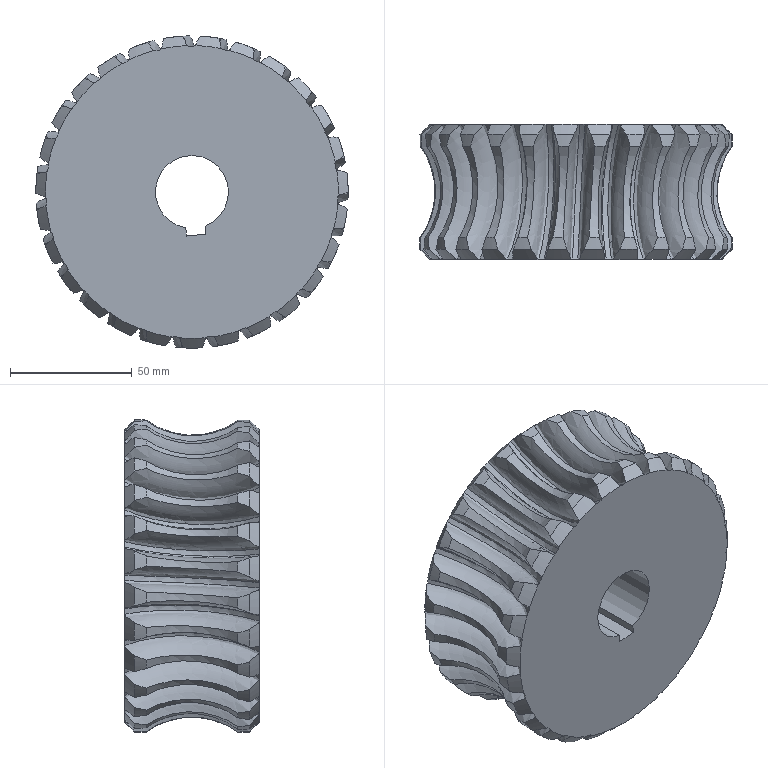Part | SolidWorks | features BaseBody 1 | 1 solid | 225 faces | box 128.363 x 55.3 x 128.358 mm | volume 529426 mm3 | spline 108 | cylinder 57 | cone 55 | plane 5 | commonest cylinder face diameters 128.363 x56 30 x1